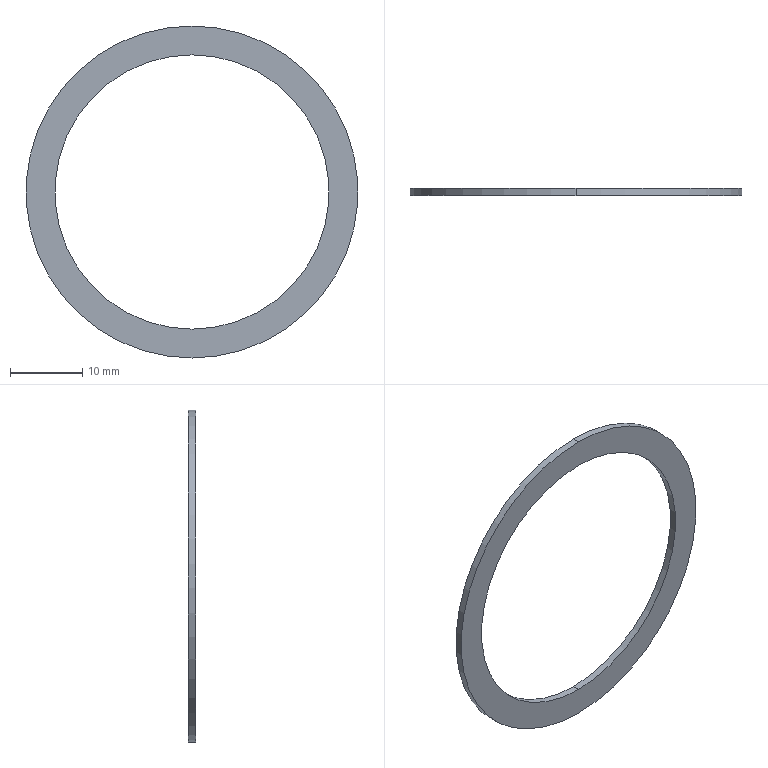Part | SolidWorks | features Revolution 1 | 1 solid | 6 faces | box 46 x 1 x 46 mm | volume 527.788 mm3 | cylinder 4 | plane 2 | commonest cylinder face diameters 38 x2 46 x2
STEP:
#1=CARTESIAN_POINT('',(0.,1.,-23.));
#2=VERTEX_POINT('',#1);
#3=CARTESIAN_POINT('',(0.,1.,23.));
#4=VERTEX_POINT('',#3);
#5=CARTESIAN_POINT('',(0.,1.,0.));
#6=DIRECTION('',(0.,-1.,0.));
#7=DIRECTION('',(0.,0.,-1.));
#8=AXIS2_PLACEMENT_3D('',#5,#6,#7);
#9=CIRCLE('',#8,23.);
#10=EDGE_CURVE('',#2,#4,#9,.T.);
#11=ORIENTED_EDGE('',*,*,#10,.T.);
#12=CARTESIAN_POINT('',(0.,0.,23.));
#13=VERTEX_POINT('',#12);
#14=CARTESIAN_POINT('',(0.,0.,23.));
#15=DIRECTION('',(0.,-1.,0.));
#16=VECTOR('',#15,1000.);
#17=LINE('',#14,#16);
#18=EDGE_CURVE('',#4,#13,#17,.T.);
#19=ORIENTED_EDGE('',*,*,#18,.T.);
#20=CARTESIAN_POINT('',(0.,0.,-23.));
#21=VERTEX_POINT('',#20);
#22=CARTESIAN_POINT('',(0.,0.,0.));
#23=DIRECTION('',(0.,-1.,0.));
#24=DIRECTION('',(0.,0.,-1.));
#25=AXIS2_PLACEMENT_3D('',#22,#23,#24);
#26=CIRCLE('',#25,23.);
#27=EDGE_CURVE('',#21,#13,#26,.T.);
#28=ORIENTED_EDGE('',*,*,#27,.F.);
#29=CARTESIAN_POINT('',(0.,0.,-23.));
#30=DIRECTION('',(0.,-1.,0.));
#31=VECTOR('',#30,1000.);
#32=LINE('',#29,#31);
#33=EDGE_CURVE('',#2,#21,#32,.T.);
#34=ORIENTED_EDGE('',*,*,#33,.F.);
#35=EDGE_LOOP('',(#11,#19,#28,#34));
#36=FACE_OUTER_BOUND('',#35,.T.);
#37=CARTESIAN_POINT('',(0.,0.,0.));
#38=DIRECTION('',(0.,-1.,0.));
#39=DIRECTION('',(0.,0.,-1.));
#40=AXIS2_PLACEMENT_3D('',#37,#38,#39);
#41=CYLINDRICAL_SURFACE('',#40,23.);
#42=ADVANCED_FACE('',(#36),#41,.T.);
#43=CARTESIAN_POINT('',(0.,1.,19.));
#44=VERTEX_POINT('',#43);
#45=CARTESIAN_POINT('',(0.,1.,-19.));
#46=VERTEX_POINT('',#45);
#47=CARTESIAN_POINT('',(0.,1.,0.));
#48=DIRECTION('',(0.,-1.,0.));
#49=DIRECTION('',(0.,0.,-1.));
#50=AXIS2_PLACEMENT_3D('',#47,#48,#49);
#51=CIRCLE('',#50,19.);
#52=EDGE_CURVE('',#44,#46,#51,.T.);
#53=ORIENTED_EDGE('',*,*,#52,.F.);
#54=CARTESIAN_POINT('',(0.,0.,19.));
#55=VERTEX_POINT('',#54);
#56=CARTESIAN_POINT('',(0.,0.,19.));
#57=DIRECTION('',(0.,-1.,0.));
#58=VECTOR('',#57,1000.);
#59=LINE('',#56,#58);
#60=EDGE_CURVE('',#44,#55,#59,.T.);
#61=ORIENTED_EDGE('',*,*,#60,.T.);
#62=CARTESIAN_POINT('',(0.,0.,-19.));
#63=VERTEX_POINT('',#62);
#64=CARTESIAN_POINT('',(0.,0.,0.));
#65=DIRECTION('',(0.,-1.,0.));
#66=DIRECTION('',(0.,0.,-1.));
#67=AXIS2_PLACEMENT_3D('',#64,#65,#66);
#68=CIRCLE('',#67,19.);
#69=EDGE_CURVE('',#55,#63,#68,.T.);
#70=ORIENTED_EDGE('',*,*,#69,.T.);
#71=CARTESIAN_POINT('',(0.,0.,-19.));
#72=DIRECTION('',(0.,-1.,0.));
#73=VECTOR('',#72,1000.);
#74=LINE('',#71,#73);
#75=EDGE_CURVE('',#46,#63,#74,.T.);
#76=ORIENTED_EDGE('',*,*,#75,.F.);
#77=EDGE_LOOP('',(#53,#61,#70,#76));
#78=FACE_OUTER_BOUND('',#77,.T.);
#79=CARTESIAN_POINT('',(0.,0.,0.));
#80=DIRECTION('',(0.,-1.,0.));
#81=DIRECTION('',(0.,0.,-1.));
#82=AXIS2_PLACEMENT_3D('',#79,#80,#81);
#83=CYLINDRICAL_SURFACE('',#82,19.);
#84=ADVANCED_FACE('',(#78),#83,.F.);
#85=ORIENTED_EDGE('',*,*,#60,.F.);
#86=CARTESIAN_POINT('',(0.,1.,0.));
#87=DIRECTION('',(0.,-1.,0.));
#88=DIRECTION('',(0.,0.,-1.));
#89=AXIS2_PLACEMENT_3D('',#86,#87,#88);
#90=CIRCLE('',#89,19.);
#91=EDGE_CURVE('',#46,#44,#90,.T.);
#92=ORIENTED_EDGE('',*,*,#91,.F.);
#93=ORIENTED_EDGE('',*,*,#75,.T.);
#94=CARTESIAN_POINT('',(0.,0.,0.));
#95=DIRECTION('',(0.,-1.,0.));
#96=DIRECTION('',(0.,0.,-1.));
#97=AXIS2_PLACEMENT_3D('',#94,#95,#96);
#98=CIRCLE('',#97,19.);
#99=EDGE_CURVE('',#63,#55,#98,.T.);
#100=ORIENTED_EDGE('',*,*,#99,.T.);
#101=EDGE_LOOP('',(#85,#92,#93,#100));
#102=FACE_OUTER_BOUND('',#101,.T.);
#103=CARTESIAN_POINT('',(0.,0.,0.));
#104=DIRECTION('',(0.,-1.,0.));
#105=DIRECTION('',(0.,0.,-1.));
#106=AXIS2_PLACEMENT_3D('',#103,#104,#105);
#107=CYLINDRICAL_SURFACE('',#106,19.);
#108=ADVANCED_FACE('',(#102),#107,.F.);
#109=ORIENTED_EDGE('',*,*,#91,.T.);
#110=ORIENTED_EDGE('',*,*,#52,.T.);
#111=EDGE_LOOP('',(#109,#110));
#112=FACE_BOUND('',#111,.T.);
#113=ORIENTED_EDGE('',*,*,#10,.F.);
#114=CARTESIAN_POINT('',(0.,1.,0.));
#115=DIRECTION('',(0.,-1.,0.));
#116=DIRECTION('',(0.,0.,-1.));
#117=AXIS2_PLACEMENT_3D('',#114,#115,#116);
#118=CIRCLE('',#117,23.);
#119=EDGE_CURVE('',#4,#2,#118,.T.);
#120=ORIENTED_EDGE('',*,*,#119,.F.);
#121=EDGE_LOOP('',(#113,#120));
#122=FACE_OUTER_BOUND('',#121,.T.);
#123=CARTESIAN_POINT('',(19.,1.,0.));
#124=DIRECTION('',(0.,1.,0.));
#125=DIRECTION('',(0.,0.,1.));
#126=AXIS2_PLACEMENT_3D('',#123,#124,#125);
#127=PLANE('',#126);
#128=ADVANCED_FACE('',(#112,#122),#127,.T.);
#129=ORIENTED_EDGE('',*,*,#18,.F.);
#130=ORIENTED_EDGE('',*,*,#119,.T.);
#131=ORIENTED_EDGE('',*,*,#33,.T.);
#132=CARTESIAN_POINT('',(0.,0.,0.));
#133=DIRECTION('',(0.,-1.,0.));
#134=DIRECTION('',(0.,0.,-1.));
#135=AXIS2_PLACEMENT_3D('',#132,#133,#134);
#136=CIRCLE('',#135,23.);
#137=EDGE_CURVE('',#13,#21,#136,.T.);
#138=ORIENTED_EDGE('',*,*,#137,.F.);
#139=EDGE_LOOP('',(#129,#130,#131,#138));
#140=FACE_OUTER_BOUND('',#139,.T.);
#141=CARTESIAN_POINT('',(0.,0.,0.));
#142=DIRECTION('',(0.,-1.,0.));
#143=DIRECTION('',(0.,0.,-1.));
#144=AXIS2_PLACEMENT_3D('',#141,#142,#143);
#145=CYLINDRICAL_SURFACE('',#144,23.);
#146=ADVANCED_FACE('',(#140),#145,.T.);
#147=ORIENTED_EDGE('',*,*,#27,.T.);
#148=ORIENTED_EDGE('',*,*,#137,.T.);
#149=EDGE_LOOP('',(#147,#148));
#150=FACE_OUTER_BOUND('',#149,.T.);
#151=ORIENTED_EDGE('',*,*,#99,.F.);
#152=ORIENTED_EDGE('',*,*,#69,.F.);
#153=EDGE_LOOP('',(#151,#152));
#154=FACE_BOUND('',#153,.T.);
#155=CARTESIAN_POINT('',(19.,0.,0.));
#156=DIRECTION('',(0.,-1.,0.));
#157=DIRECTION('',(0.,0.,-1.));
#158=AXIS2_PLACEMENT_3D('',#155,#156,#157);
#159=PLANE('',#158);
#160=ADVANCED_FACE('',(#150,#154),#159,.T.);
#161=CLOSED_SHELL('',(#42,#84,#108,#128,#146,#160));
#162=MANIFOLD_SOLID_BREP('',#161);
#163=CARTESIAN_POINT('',(0.,0.,0.));
#164=DIRECTION('',(0.,0.,1.));
#165=DIRECTION('',(1.,0.,0.));
#166=AXIS2_PLACEMENT_3D('',#163,#164,#165);
#167=(LENGTH_UNIT()NAMED_UNIT(*)SI_UNIT(.MILLI.,.METRE.));
#168=UNCERTAINTY_MEASURE_WITH_UNIT(LENGTH_MEASURE(0.00001),#167,'','');
#169=(NAMED_UNIT(*)PLANE_ANGLE_UNIT()SI_UNIT($,.RADIAN.));
#170=(NAMED_UNIT(*)SI_UNIT($,.STERADIAN.)SOLID_ANGLE_UNIT());
#171=(GEOMETRIC_REPRESENTATION_CONTEXT(3)GLOBAL_UNCERTAINTY_ASSIGNED_CONTEXT((#168))GLOBAL_UNIT_ASSIGNED_CONTEXT((#167,#169,#170))REPRESENTATION_CONTEXT('',''));
#172=ADVANCED_BREP_SHAPE_REPRESENTATION('',(#162,#166),#171);